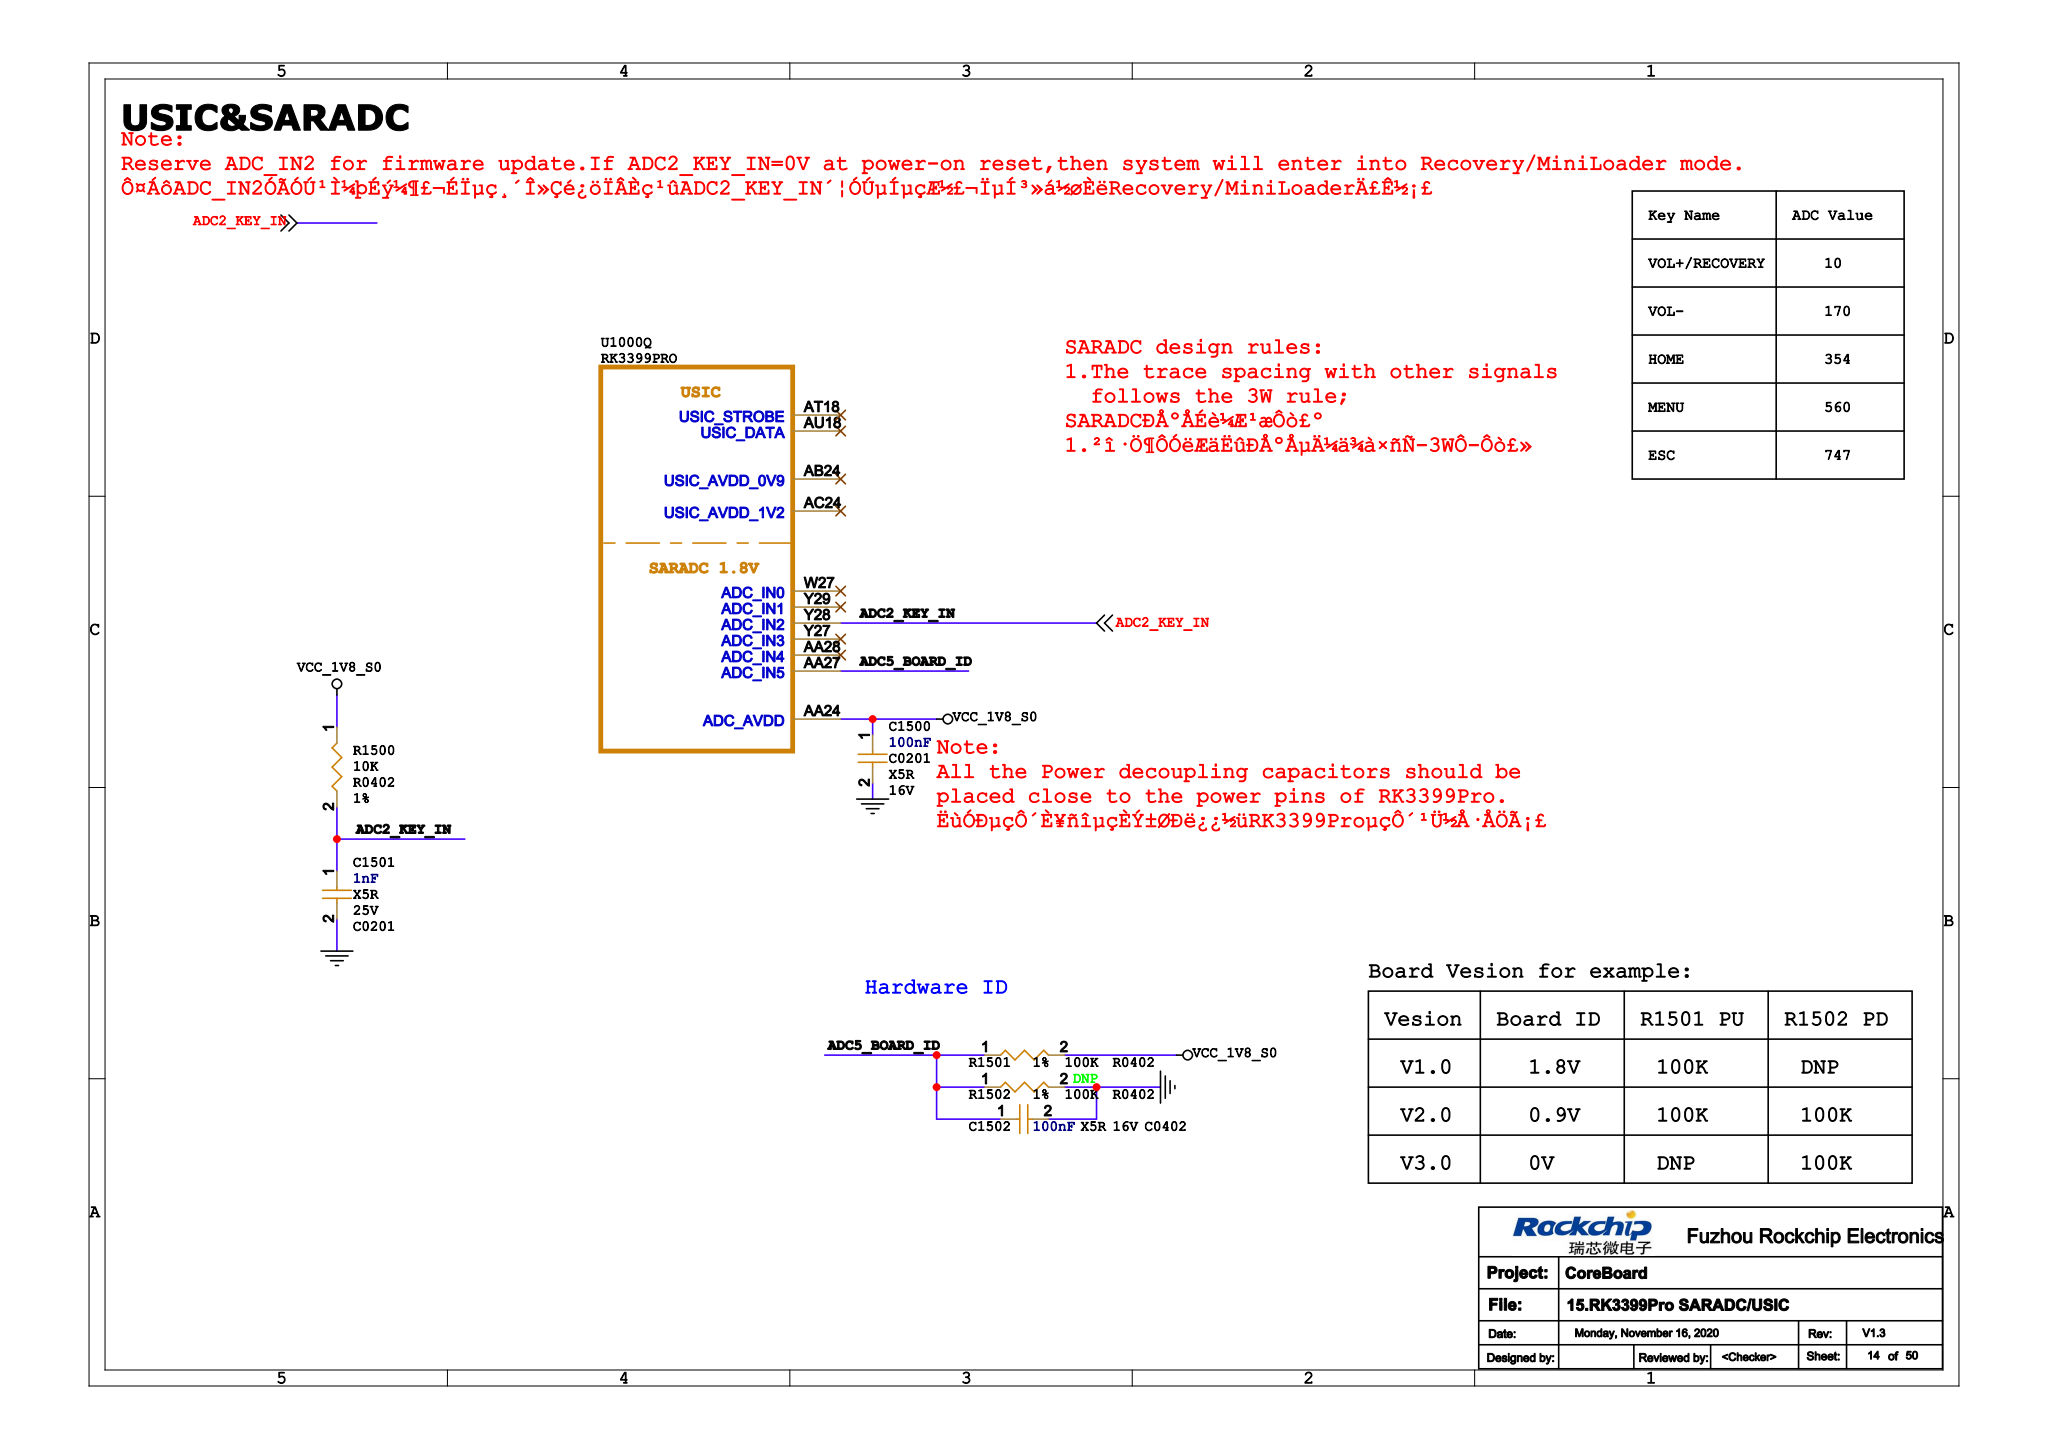Circuit board | Cadence Allegro | 749 parts | 717 nets | one sheet of the schematic
Parts on this sheet (reference | value | footprint):
C1500 | 100nF | C0201
C1501 | 1nF | C0201
C1502 | 100nF | C0402
R1500 | 10K | R0402
R1501 | 100K | R0402
R1502 | 100K | R0402
Nets of these parts (net: part-pin ...):
GND: C1500-2 C1501-2 C1502-2 R1502-2
VCC_1V8_S0: C1500-1 R1500-1 R1501-2
ADC2_KEY_IN: C1501-1 R1500-2
ADC5_BOARD_ID: C1502-1 R1501-1 R1502-1